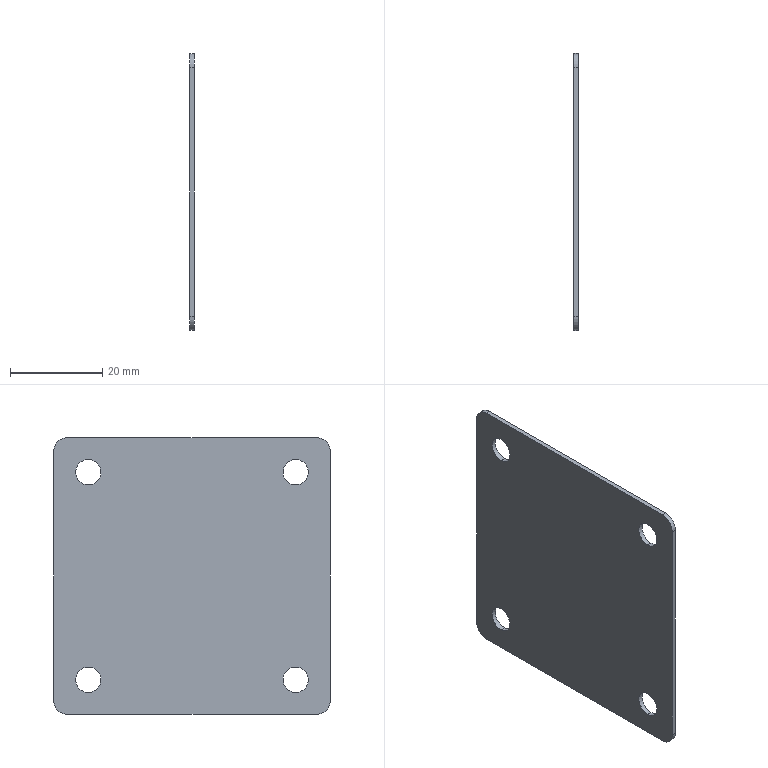Part | STEP file | FFH80-GY-022^FFH85-B3 -02_three-axis module | 1 solid | 18 faces | box 1 x 60 x 60 mm | volume 3497 mm3 | cylinder 12 | plane 6 | commonest cylinder face diameters 5.5 x8 6 x4
STEP:
#1=CARTESIAN_POINT('',(0.,22.5,-19.75));
#2=VERTEX_POINT('',#1);
#3=CARTESIAN_POINT('',(0.,22.5,-25.25));
#4=VERTEX_POINT('',#3);
#5=CARTESIAN_POINT('',(0.,22.5,-22.5));
#6=DIRECTION('',(1.,0.,0.));
#7=DIRECTION('',(0.,0.,-1.));
#8=AXIS2_PLACEMENT_3D('',#5,#6,#7);
#9=CIRCLE('',#8,2.75);
#10=EDGE_CURVE('',#2,#4,#9,.T.);
#11=ORIENTED_EDGE('',*,*,#10,.F.);
#12=CARTESIAN_POINT('',(1.,22.5,-19.75));
#13=VERTEX_POINT('',#12);
#14=CARTESIAN_POINT('',(1.,22.5,-19.75));
#15=DIRECTION('',(1.,0.,0.));
#16=VECTOR('',#15,1000.);
#17=LINE('',#14,#16);
#18=EDGE_CURVE('',#2,#13,#17,.T.);
#19=ORIENTED_EDGE('',*,*,#18,.T.);
#20=CARTESIAN_POINT('',(1.,22.5,-25.25));
#21=VERTEX_POINT('',#20);
#22=CARTESIAN_POINT('',(1.,22.5,-22.5));
#23=DIRECTION('',(1.,0.,0.));
#24=DIRECTION('',(0.,0.,-1.));
#25=AXIS2_PLACEMENT_3D('',#22,#23,#24);
#26=CIRCLE('',#25,2.75);
#27=EDGE_CURVE('',#13,#21,#26,.T.);
#28=ORIENTED_EDGE('',*,*,#27,.T.);
#29=CARTESIAN_POINT('',(1.,22.5,-25.25));
#30=DIRECTION('',(1.,0.,0.));
#31=VECTOR('',#30,1000.);
#32=LINE('',#29,#31);
#33=EDGE_CURVE('',#4,#21,#32,.T.);
#34=ORIENTED_EDGE('',*,*,#33,.F.);
#35=EDGE_LOOP('',(#11,#19,#28,#34));
#36=FACE_OUTER_BOUND('',#35,.T.);
#37=CARTESIAN_POINT('',(1.,22.5,-22.5));
#38=DIRECTION('',(1.,0.,0.));
#39=DIRECTION('',(0.,0.,-1.));
#40=AXIS2_PLACEMENT_3D('',#37,#38,#39);
#41=CYLINDRICAL_SURFACE('',#40,2.75);
#42=ADVANCED_FACE('',(#36),#41,.F.);
#43=CARTESIAN_POINT('',(0.,22.5,25.25));
#44=VERTEX_POINT('',#43);
#45=CARTESIAN_POINT('',(0.,22.5,19.75));
#46=VERTEX_POINT('',#45);
#47=CARTESIAN_POINT('',(0.,22.5,22.5));
#48=DIRECTION('',(1.,0.,0.));
#49=DIRECTION('',(0.,0.,-1.));
#50=AXIS2_PLACEMENT_3D('',#47,#48,#49);
#51=CIRCLE('',#50,2.75);
#52=EDGE_CURVE('',#44,#46,#51,.T.);
#53=ORIENTED_EDGE('',*,*,#52,.F.);
#54=CARTESIAN_POINT('',(1.,22.5,25.25));
#55=VERTEX_POINT('',#54);
#56=CARTESIAN_POINT('',(1.,22.5,25.25));
#57=DIRECTION('',(1.,0.,0.));
#58=VECTOR('',#57,1000.);
#59=LINE('',#56,#58);
#60=EDGE_CURVE('',#44,#55,#59,.T.);
#61=ORIENTED_EDGE('',*,*,#60,.T.);
#62=CARTESIAN_POINT('',(1.,22.5,19.75));
#63=VERTEX_POINT('',#62);
#64=CARTESIAN_POINT('',(1.,22.5,22.5));
#65=DIRECTION('',(1.,0.,0.));
#66=DIRECTION('',(0.,0.,-1.));
#67=AXIS2_PLACEMENT_3D('',#64,#65,#66);
#68=CIRCLE('',#67,2.75);
#69=EDGE_CURVE('',#55,#63,#68,.T.);
#70=ORIENTED_EDGE('',*,*,#69,.T.);
#71=CARTESIAN_POINT('',(1.,22.5,19.75));
#72=DIRECTION('',(1.,0.,0.));
#73=VECTOR('',#72,1000.);
#74=LINE('',#71,#73);
#75=EDGE_CURVE('',#46,#63,#74,.T.);
#76=ORIENTED_EDGE('',*,*,#75,.F.);
#77=EDGE_LOOP('',(#53,#61,#70,#76));
#78=FACE_OUTER_BOUND('',#77,.T.);
#79=CARTESIAN_POINT('',(1.,22.5,22.5));
#80=DIRECTION('',(1.,0.,0.));
#81=DIRECTION('',(0.,0.,-1.));
#82=AXIS2_PLACEMENT_3D('',#79,#80,#81);
#83=CYLINDRICAL_SURFACE('',#82,2.75);
#84=ADVANCED_FACE('',(#78),#83,.F.);
#85=CARTESIAN_POINT('',(0.,-22.5,-19.75));
#86=VERTEX_POINT('',#85);
#87=CARTESIAN_POINT('',(0.,-22.5,-25.25));
#88=VERTEX_POINT('',#87);
#89=CARTESIAN_POINT('',(0.,-22.5,-22.5));
#90=DIRECTION('',(1.,0.,0.));
#91=DIRECTION('',(0.,0.,-1.));
#92=AXIS2_PLACEMENT_3D('',#89,#90,#91);
#93=CIRCLE('',#92,2.75);
#94=EDGE_CURVE('',#86,#88,#93,.T.);
#95=ORIENTED_EDGE('',*,*,#94,.F.);
#96=CARTESIAN_POINT('',(1.,-22.5,-19.75));
#97=VERTEX_POINT('',#96);
#98=CARTESIAN_POINT('',(1.,-22.5,-19.75));
#99=DIRECTION('',(1.,0.,0.));
#100=VECTOR('',#99,1000.);
#101=LINE('',#98,#100);
#102=EDGE_CURVE('',#86,#97,#101,.T.);
#103=ORIENTED_EDGE('',*,*,#102,.T.);
#104=CARTESIAN_POINT('',(1.,-22.5,-25.25));
#105=VERTEX_POINT('',#104);
#106=CARTESIAN_POINT('',(1.,-22.5,-22.5));
#107=DIRECTION('',(1.,0.,0.));
#108=DIRECTION('',(0.,0.,-1.));
#109=AXIS2_PLACEMENT_3D('',#106,#107,#108);
#110=CIRCLE('',#109,2.75);
#111=EDGE_CURVE('',#97,#105,#110,.T.);
#112=ORIENTED_EDGE('',*,*,#111,.T.);
#113=CARTESIAN_POINT('',(1.,-22.5,-25.25));
#114=DIRECTION('',(1.,0.,0.));
#115=VECTOR('',#114,1000.);
#116=LINE('',#113,#115);
#117=EDGE_CURVE('',#88,#105,#116,.T.);
#118=ORIENTED_EDGE('',*,*,#117,.F.);
#119=EDGE_LOOP('',(#95,#103,#112,#118));
#120=FACE_OUTER_BOUND('',#119,.T.);
#121=CARTESIAN_POINT('',(1.,-22.5,-22.5));
#122=DIRECTION('',(1.,0.,0.));
#123=DIRECTION('',(0.,0.,-1.));
#124=AXIS2_PLACEMENT_3D('',#121,#122,#123);
#125=CYLINDRICAL_SURFACE('',#124,2.75);
#126=ADVANCED_FACE('',(#120),#125,.F.);
#127=CARTESIAN_POINT('',(0.,-22.5,25.25));
#128=VERTEX_POINT('',#127);
#129=CARTESIAN_POINT('',(0.,-22.5,19.75));
#130=VERTEX_POINT('',#129);
#131=CARTESIAN_POINT('',(0.,-22.5,22.5));
#132=DIRECTION('',(1.,0.,0.));
#133=DIRECTION('',(0.,0.,-1.));
#134=AXIS2_PLACEMENT_3D('',#131,#132,#133);
#135=CIRCLE('',#134,2.75);
#136=EDGE_CURVE('',#128,#130,#135,.T.);
#137=ORIENTED_EDGE('',*,*,#136,.F.);
#138=CARTESIAN_POINT('',(1.,-22.5,25.25));
#139=VERTEX_POINT('',#138);
#140=CARTESIAN_POINT('',(1.,-22.5,25.25));
#141=DIRECTION('',(1.,0.,0.));
#142=VECTOR('',#141,1000.);
#143=LINE('',#140,#142);
#144=EDGE_CURVE('',#128,#139,#143,.T.);
#145=ORIENTED_EDGE('',*,*,#144,.T.);
#146=CARTESIAN_POINT('',(1.,-22.5,19.75));
#147=VERTEX_POINT('',#146);
#148=CARTESIAN_POINT('',(1.,-22.5,22.5));
#149=DIRECTION('',(1.,0.,0.));
#150=DIRECTION('',(0.,0.,-1.));
#151=AXIS2_PLACEMENT_3D('',#148,#149,#150);
#152=CIRCLE('',#151,2.75);
#153=EDGE_CURVE('',#139,#147,#152,.T.);
#154=ORIENTED_EDGE('',*,*,#153,.T.);
#155=CARTESIAN_POINT('',(1.,-22.5,19.75));
#156=DIRECTION('',(1.,0.,0.));
#157=VECTOR('',#156,1000.);
#158=LINE('',#155,#157);
#159=EDGE_CURVE('',#130,#147,#158,.T.);
#160=ORIENTED_EDGE('',*,*,#159,.F.);
#161=EDGE_LOOP('',(#137,#145,#154,#160));
#162=FACE_OUTER_BOUND('',#161,.T.);
#163=CARTESIAN_POINT('',(1.,-22.5,22.5));
#164=DIRECTION('',(1.,0.,0.));
#165=DIRECTION('',(0.,0.,-1.));
#166=AXIS2_PLACEMENT_3D('',#163,#164,#165);
#167=CYLINDRICAL_SURFACE('',#166,2.75);
#168=ADVANCED_FACE('',(#162),#167,.F.);
#169=CARTESIAN_POINT('',(1.,22.5,-22.5));
#170=DIRECTION('',(1.,0.,0.));
#171=DIRECTION('',(0.,0.,-1.));
#172=AXIS2_PLACEMENT_3D('',#169,#170,#171);
#173=CIRCLE('',#172,2.75);
#174=EDGE_CURVE('',#21,#13,#173,.T.);
#175=ORIENTED_EDGE('',*,*,#174,.F.);
#176=ORIENTED_EDGE('',*,*,#27,.F.);
#177=EDGE_LOOP('',(#175,#176));
#178=FACE_BOUND('',#177,.T.);
#179=CARTESIAN_POINT('',(1.,22.5,22.5));
#180=DIRECTION('',(1.,0.,0.));
#181=DIRECTION('',(0.,0.,-1.));
#182=AXIS2_PLACEMENT_3D('',#179,#180,#181);
#183=CIRCLE('',#182,2.75);
#184=EDGE_CURVE('',#63,#55,#183,.T.);
#185=ORIENTED_EDGE('',*,*,#184,.F.);
#186=ORIENTED_EDGE('',*,*,#69,.F.);
#187=EDGE_LOOP('',(#185,#186));
#188=FACE_BOUND('',#187,.T.);
#189=CARTESIAN_POINT('',(1.,-22.5,-22.5));
#190=DIRECTION('',(1.,0.,0.));
#191=DIRECTION('',(0.,0.,-1.));
#192=AXIS2_PLACEMENT_3D('',#189,#190,#191);
#193=CIRCLE('',#192,2.75);
#194=EDGE_CURVE('',#105,#97,#193,.T.);
#195=ORIENTED_EDGE('',*,*,#194,.F.);
#196=ORIENTED_EDGE('',*,*,#111,.F.);
#197=EDGE_LOOP('',(#195,#196));
#198=FACE_BOUND('',#197,.T.);
#199=CARTESIAN_POINT('',(1.,-22.5,22.5));
#200=DIRECTION('',(1.,0.,0.));
#201=DIRECTION('',(0.,0.,-1.));
#202=AXIS2_PLACEMENT_3D('',#199,#200,#201);
#203=CIRCLE('',#202,2.75);
#204=EDGE_CURVE('',#147,#139,#203,.T.);
#205=ORIENTED_EDGE('',*,*,#204,.F.);
#206=ORIENTED_EDGE('',*,*,#153,.F.);
#207=EDGE_LOOP('',(#205,#206));
#208=FACE_BOUND('',#207,.T.);
#209=CARTESIAN_POINT('',(1.,-30.,-27.));
#210=VERTEX_POINT('',#209);
#211=CARTESIAN_POINT('',(1.,-30.,27.));
#212=VERTEX_POINT('',#211);
#213=CARTESIAN_POINT('',(1.,-30.,0.));
#214=DIRECTION('',(0.,0.,1.));
#215=VECTOR('',#214,1000.);
#216=LINE('',#213,#215);
#217=EDGE_CURVE('',#210,#212,#216,.T.);
#218=ORIENTED_EDGE('',*,*,#217,.F.);
#219=CARTESIAN_POINT('',(1.,-27.,-30.));
#220=VERTEX_POINT('',#219);
#221=CARTESIAN_POINT('',(1.,-27.,-27.));
#222=DIRECTION('',(-1.,0.,0.));
#223=DIRECTION('',(0.,0.,1.));
#224=AXIS2_PLACEMENT_3D('',#221,#222,#223);
#225=CIRCLE('',#224,3.);
#226=EDGE_CURVE('',#220,#210,#225,.T.);
#227=ORIENTED_EDGE('',*,*,#226,.F.);
#228=CARTESIAN_POINT('',(1.,27.,-30.));
#229=VERTEX_POINT('',#228);
#230=CARTESIAN_POINT('',(1.,0.,-30.));
#231=DIRECTION('',(0.,-1.,0.));
#232=VECTOR('',#231,1000.);
#233=LINE('',#230,#232);
#234=EDGE_CURVE('',#229,#220,#233,.T.);
#235=ORIENTED_EDGE('',*,*,#234,.F.);
#236=CARTESIAN_POINT('',(1.,30.,-27.));
#237=VERTEX_POINT('',#236);
#238=CARTESIAN_POINT('',(1.,27.,-27.));
#239=DIRECTION('',(-1.,0.,0.));
#240=DIRECTION('',(0.,0.,1.));
#241=AXIS2_PLACEMENT_3D('',#238,#239,#240);
#242=CIRCLE('',#241,3.);
#243=EDGE_CURVE('',#237,#229,#242,.T.);
#244=ORIENTED_EDGE('',*,*,#243,.F.);
#245=CARTESIAN_POINT('',(1.,30.,27.));
#246=VERTEX_POINT('',#245);
#247=CARTESIAN_POINT('',(1.,30.,0.));
#248=DIRECTION('',(0.,0.,-1.));
#249=VECTOR('',#248,1000.);
#250=LINE('',#247,#249);
#251=EDGE_CURVE('',#246,#237,#250,.T.);
#252=ORIENTED_EDGE('',*,*,#251,.F.);
#253=CARTESIAN_POINT('',(1.,27.,30.));
#254=VERTEX_POINT('',#253);
#255=CARTESIAN_POINT('',(1.,27.,27.));
#256=DIRECTION('',(-1.,0.,0.));
#257=DIRECTION('',(0.,0.,1.));
#258=AXIS2_PLACEMENT_3D('',#255,#256,#257);
#259=CIRCLE('',#258,3.);
#260=EDGE_CURVE('',#254,#246,#259,.T.);
#261=ORIENTED_EDGE('',*,*,#260,.F.);
#262=CARTESIAN_POINT('',(1.,-27.,30.));
#263=VERTEX_POINT('',#262);
#264=CARTESIAN_POINT('',(1.,0.,30.));
#265=DIRECTION('',(0.,1.,0.));
#266=VECTOR('',#265,1000.);
#267=LINE('',#264,#266);
#268=EDGE_CURVE('',#263,#254,#267,.T.);
#269=ORIENTED_EDGE('',*,*,#268,.F.);
#270=CARTESIAN_POINT('',(1.,-27.,27.));
#271=DIRECTION('',(-1.,0.,0.));
#272=DIRECTION('',(0.,0.,1.));
#273=AXIS2_PLACEMENT_3D('',#270,#271,#272);
#274=CIRCLE('',#273,3.);
#275=EDGE_CURVE('',#212,#263,#274,.T.);
#276=ORIENTED_EDGE('',*,*,#275,.F.);
#277=EDGE_LOOP('',(#218,#227,#235,#244,#252,#261,#269,#276));
#278=FACE_OUTER_BOUND('',#277,.T.);
#279=CARTESIAN_POINT('',(1.,0.,0.));
#280=DIRECTION('',(-1.,0.,0.));
#281=DIRECTION('',(0.,0.,1.));
#282=AXIS2_PLACEMENT_3D('',#279,#280,#281);
#283=PLANE('',#282);
#284=ADVANCED_FACE('',(#178,#188,#198,#208,#278),#283,.F.);
#285=ORIENTED_EDGE('',*,*,#18,.F.);
#286=CARTESIAN_POINT('',(0.,22.5,-22.5));
#287=DIRECTION('',(1.,0.,0.));
#288=DIRECTION('',(0.,0.,-1.));
#289=AXIS2_PLACEMENT_3D('',#286,#287,#288);
#290=CIRCLE('',#289,2.75);
#291=EDGE_CURVE('',#4,#2,#290,.T.);
#292=ORIENTED_EDGE('',*,*,#291,.F.);
#293=ORIENTED_EDGE('',*,*,#33,.T.);
#294=ORIENTED_EDGE('',*,*,#174,.T.);
#295=EDGE_LOOP('',(#285,#292,#293,#294));
#296=FACE_OUTER_BOUND('',#295,.T.);
#297=CARTESIAN_POINT('',(1.,22.5,-22.5));
#298=DIRECTION('',(1.,0.,0.));
#299=DIRECTION('',(0.,0.,-1.));
#300=AXIS2_PLACEMENT_3D('',#297,#298,#299);
#301=CYLINDRICAL_SURFACE('',#300,2.75);
#302=ADVANCED_FACE('',(#296),#301,.F.);
#303=ORIENTED_EDGE('',*,*,#60,.F.);
#304=CARTESIAN_POINT('',(0.,22.5,22.5));
#305=DIRECTION('',(1.,0.,0.));
#306=DIRECTION('',(0.,0.,-1.));
#307=AXIS2_PLACEMENT_3D('',#304,#305,#306);
#308=CIRCLE('',#307,2.75);
#309=EDGE_CURVE('',#46,#44,#308,.T.);
#310=ORIENTED_EDGE('',*,*,#309,.F.);
#311=ORIENTED_EDGE('',*,*,#75,.T.);
#312=ORIENTED_EDGE('',*,*,#184,.T.);
#313=EDGE_LOOP('',(#303,#310,#311,#312));
#314=FACE_OUTER_BOUND('',#313,.T.);
#315=CARTESIAN_POINT('',(1.,22.5,22.5));
#316=DIRECTION('',(1.,0.,0.));
#317=DIRECTION('',(0.,0.,-1.));
#318=AXIS2_PLACEMENT_3D('',#315,#316,#317);
#319=CYLINDRICAL_SURFACE('',#318,2.75);
#320=ADVANCED_FACE('',(#314),#319,.F.);
#321=ORIENTED_EDGE('',*,*,#102,.F.);
#322=CARTESIAN_POINT('',(0.,-22.5,-22.5));
#323=DIRECTION('',(1.,0.,0.));
#324=DIRECTION('',(0.,0.,-1.));
#325=AXIS2_PLACEMENT_3D('',#322,#323,#324);
#326=CIRCLE('',#325,2.75);
#327=EDGE_CURVE('',#88,#86,#326,.T.);
#328=ORIENTED_EDGE('',*,*,#327,.F.);
#329=ORIENTED_EDGE('',*,*,#117,.T.);
#330=ORIENTED_EDGE('',*,*,#194,.T.);
#331=EDGE_LOOP('',(#321,#328,#329,#330));
#332=FACE_OUTER_BOUND('',#331,.T.);
#333=CARTESIAN_POINT('',(1.,-22.5,-22.5));
#334=DIRECTION('',(1.,0.,0.));
#335=DIRECTION('',(0.,0.,-1.));
#336=AXIS2_PLACEMENT_3D('',#333,#334,#335);
#337=CYLINDRICAL_SURFACE('',#336,2.75);
#338=ADVANCED_FACE('',(#332),#337,.F.);
#339=ORIENTED_EDGE('',*,*,#144,.F.);
#340=CARTESIAN_POINT('',(0.,-22.5,22.5));
#341=DIRECTION('',(1.,0.,0.));
#342=DIRECTION('',(0.,0.,-1.));
#343=AXIS2_PLACEMENT_3D('',#340,#341,#342);
#344=CIRCLE('',#343,2.75);
#345=EDGE_CURVE('',#130,#128,#344,.T.);
#346=ORIENTED_EDGE('',*,*,#345,.F.);
#347=ORIENTED_EDGE('',*,*,#159,.T.);
#348=ORIENTED_EDGE('',*,*,#204,.T.);
#349=EDGE_LOOP('',(#339,#346,#347,#348));
#350=FACE_OUTER_BOUND('',#349,.T.);
#351=CARTESIAN_POINT('',(1.,-22.5,22.5));
#352=DIRECTION('',(1.,0.,0.));
#353=DIRECTION('',(0.,0.,-1.));
#354=AXIS2_PLACEMENT_3D('',#351,#352,#353);
#355=CYLINDRICAL_SURFACE('',#354,2.75);
#356=ADVANCED_FACE('',(#350),#355,.F.);
#357=ORIENTED_EDGE('',*,*,#275,.T.);
#358=CARTESIAN_POINT('',(0.,-27.,30.));
#359=VERTEX_POINT('',#358);
#360=CARTESIAN_POINT('',(1.,-27.,30.));
#361=DIRECTION('',(-1.,0.,0.));
#362=VECTOR('',#361,1000.);
#363=LINE('',#360,#362);
#364=EDGE_CURVE('',#263,#359,#363,.T.);
#365=ORIENTED_EDGE('',*,*,#364,.T.);
#366=CARTESIAN_POINT('',(0.,-30.,27.));
#367=VERTEX_POINT('',#366);
#368=CARTESIAN_POINT('',(0.,-27.,27.));
#369=DIRECTION('',(1.,0.,0.));
#370=DIRECTION('',(0.,0.,1.));
#371=AXIS2_PLACEMENT_3D('',#368,#369,#370);
#372=CIRCLE('',#371,3.);
#373=EDGE_CURVE('',#359,#367,#372,.T.);
#374=ORIENTED_EDGE('',*,*,#373,.T.);
#375=CARTESIAN_POINT('',(1.,-30.,27.));
#376=DIRECTION('',(1.,0.,0.));
#377=VECTOR('',#376,1000.);
#378=LINE('',#375,#377);
#379=EDGE_CURVE('',#367,#212,#378,.T.);
#380=ORIENTED_EDGE('',*,*,#379,.T.);
#381=EDGE_LOOP('',(#357,#365,#374,#380));
#382=FACE_OUTER_BOUND('',#381,.T.);
#383=CARTESIAN_POINT('',(1.,-27.,27.));
#384=DIRECTION('',(-1.,0.,0.));
#385=DIRECTION('',(0.,0.,1.));
#386=AXIS2_PLACEMENT_3D('',#383,#384,#385);
#387=CYLINDRICAL_SURFACE('',#386,3.);
#388=ADVANCED_FACE('',(#382),#387,.T.);
#389=CARTESIAN_POINT('',(0.,-30.,-27.));
#390=VERTEX_POINT('',#389);
#391=CARTESIAN_POINT('',(0.,-30.,-30.));
#392=DIRECTION('',(0.,0.,1.));
#393=VECTOR('',#392,1000.);
#394=LINE('',#391,#393);
#395=EDGE_CURVE('',#390,#367,#394,.T.);
#396=ORIENTED_EDGE('',*,*,#395,.F.);
#397=CARTESIAN_POINT('',(1.,-30.,-27.));
#398=DIRECTION('',(-1.,0.,0.));
#399=VECTOR('',#398,1000.);
#400=LINE('',#397,#399);
#401=EDGE_CURVE('',#210,#390,#400,.T.);
#402=ORIENTED_EDGE('',*,*,#401,.F.);
#403=ORIENTED_EDGE('',*,*,#217,.T.);
#404=ORIENTED_EDGE('',*,*,#379,.F.);
#405=EDGE_LOOP('',(#396,#402,#403,#404));
#406=FACE_OUTER_BOUND('',#405,.T.);
#407=CARTESIAN_POINT('',(1.,-30.,-30.));
#408=DIRECTION('',(0.,1.,0.));
#409=DIRECTION('',(0.,0.,1.));
#410=AXIS2_PLACEMENT_3D('',#407,#408,#409);
#411=PLANE('',#410);
#412=ADVANCED_FACE('',(#406),#411,.F.);
#413=ORIENTED_EDGE('',*,*,#226,.T.);
#414=ORIENTED_EDGE('',*,*,#401,.T.);
#415=CARTESIAN_POINT('',(0.,-27.,-30.));
#416=VERTEX_POINT('',#415);
#417=CARTESIAN_POINT('',(0.,-27.,-27.));
#418=DIRECTION('',(1.,0.,0.));
#419=DIRECTION('',(0.,0.,1.));
#420=AXIS2_PLACEMENT_3D('',#417,#418,#419);
#421=CIRCLE('',#420,3.);
#422=EDGE_CURVE('',#390,#416,#421,.T.);
#423=ORIENTED_EDGE('',*,*,#422,.T.);
#424=CARTESIAN_POINT('',(1.,-27.,-30.));
#425=DIRECTION('',(1.,0.,0.));
#426=VECTOR('',#425,1000.);
#427=LINE('',#424,#426);
#428=EDGE_CURVE('',#416,#220,#427,.T.);
#429=ORIENTED_EDGE('',*,*,#428,.T.);
#430=EDGE_LOOP('',(#413,#414,#423,#429));
#431=FACE_OUTER_BOUND('',#430,.T.);
#432=CARTESIAN_POINT('',(1.,-27.,-27.));
#433=DIRECTION('',(-1.,0.,0.));
#434=DIRECTION('',(0.,0.,1.));
#435=AXIS2_PLACEMENT_3D('',#432,#433,#434);
#436=CYLINDRICAL_SURFACE('',#435,3.);
#437=ADVANCED_FACE('',(#431),#436,.T.);
#438=CARTESIAN_POINT('',(0.,27.,-30.));
#439=VERTEX_POINT('',#438);
#440=CARTESIAN_POINT('',(0.,30.,-30.));
#441=DIRECTION('',(0.,-1.,0.));
#442=VECTOR('',#441,1000.);
#443=LINE('',#440,#442);
#444=EDGE_CURVE('',#439,#416,#443,.T.);
#445=ORIENTED_EDGE('',*,*,#444,.F.);
#446=CARTESIAN_POINT('',(1.,27.,-30.));
#447=DIRECTION('',(-1.,0.,0.));
#448=VECTOR('',#447,1000.);
#449=LINE('',#446,#448);
#450=EDGE_CURVE('',#229,#439,#449,.T.);
#451=ORIENTED_EDGE('',*,*,#450,.F.);
#452=ORIENTED_EDGE('',*,*,#234,.T.);
#453=ORIENTED_EDGE('',*,*,#428,.F.);
#454=EDGE_LOOP('',(#445,#451,#452,#453));
#455=FACE_OUTER_BOUND('',#454,.T.);
#456=CARTESIAN_POINT('',(1.,30.,-30.));
#457=DIRECTION('',(0.,0.,1.));
#458=DIRECTION('',(0.,-1.,0.));
#459=AXIS2_PLACEMENT_3D('',#456,#457,#458);
#460=PLANE('',#459);
#461=ADVANCED_FACE('',(#455),#460,.F.);
#462=ORIENTED_EDGE('',*,*,#243,.T.);
#463=ORIENTED_EDGE('',*,*,#450,.T.);
#464=CARTESIAN_POINT('',(0.,30.,-27.));
#465=VERTEX_POINT('',#464);
#466=CARTESIAN_POINT('',(0.,27.,-27.));
#467=DIRECTION('',(1.,0.,0.));
#468=DIRECTION('',(0.,0.,1.));
#469=AXIS2_PLACEMENT_3D('',#466,#467,#468);
#470=CIRCLE('',#469,3.);
#471=EDGE_CURVE('',#439,#465,#470,.T.);
#472=ORIENTED_EDGE('',*,*,#471,.T.);
#473=CARTESIAN_POINT('',(1.,30.,-27.));
#474=DIRECTION('',(1.,0.,0.));
#475=VECTOR('',#474,1000.);
#476=LINE('',#473,#475);
#477=EDGE_CURVE('',#465,#237,#476,.T.);
#478=ORIENTED_EDGE('',*,*,#477,.T.);
#479=EDGE_LOOP('',(#462,#463,#472,#478));
#480=FACE_OUTER_BOUND('',#479,.T.);
#481=CARTESIAN_POINT('',(1.,27.,-27.));
#482=DIRECTION('',(-1.,0.,0.));
#483=DIRECTION('',(0.,0.,1.));
#484=AXIS2_PLACEMENT_3D('',#481,#482,#483);
#485=CYLINDRICAL_SURFACE('',#484,3.);
#486=ADVANCED_FACE('',(#480),#485,.T.);
#487=CARTESIAN_POINT('',(0.,30.,27.));
#488=VERTEX_POINT('',#487);
#489=CARTESIAN_POINT('',(0.,30.,-30.));
#490=DIRECTION('',(0.,0.,-1.));
#491=VECTOR('',#490,1000.);
#492=LINE('',#489,#491);
#493=EDGE_CURVE('',#488,#465,#492,.T.);
#494=ORIENTED_EDGE('',*,*,#493,.F.);
#495=CARTESIAN_POINT('',(1.,30.,27.));
#496=DIRECTION('',(-1.,0.,0.));
#497=VECTOR('',#496,1000.);
#498=LINE('',#495,#497);
#499=EDGE_CURVE('',#246,#488,#498,.T.);
#500=ORIENTED_EDGE('',*,*,#499,.F.);
#501=ORIENTED_EDGE('',*,*,#251,.T.);
#502=ORIENTED_EDGE('',*,*,#477,.F.);
#503=EDGE_LOOP('',(#494,#500,#501,#502));
#504=FACE_OUTER_BOUND('',#503,.T.);
#505=CARTESIAN_POINT('',(1.,30.,-30.));
#506=DIRECTION('',(0.,-1.,0.));
#507=DIRECTION('',(0.,0.,-1.));
#508=AXIS2_PLACEMENT_3D('',#505,#506,#507);
#509=PLANE('',#508);
#510=ADVANCED_FACE('',(#504),#509,.F.);
#511=ORIENTED_EDGE('',*,*,#260,.T.);
#512=ORIENTED_EDGE('',*,*,#499,.T.);
#513=CARTESIAN_POINT('',(0.,27.,30.));
#514=VERTEX_POINT('',#513);
#515=CARTESIAN_POINT('',(0.,27.,27.));
#516=DIRECTION('',(1.,0.,0.));
#517=DIRECTION('',(0.,0.,1.));
#518=AXIS2_PLACEMENT_3D('',#515,#516,#517);
#519=CIRCLE('',#518,3.);
#520=EDGE_CURVE('',#488,#514,#519,.T.);
#521=ORIENTED_EDGE('',*,*,#520,.T.);
#522=CARTESIAN_POINT('',(1.,27.,30.));
#523=DIRECTION('',(1.,0.,0.));
#524=VECTOR('',#523,1000.);
#525=LINE('',#522,#524);
#526=EDGE_CURVE('',#514,#254,#525,.T.);
#527=ORIENTED_EDGE('',*,*,#526,.T.);
#528=EDGE_LOOP('',(#511,#512,#521,#527));
#529=FACE_OUTER_BOUND('',#528,.T.);
#530=CARTESIAN_POINT('',(1.,27.,27.));
#531=DIRECTION('',(-1.,0.,0.));
#532=DIRECTION('',(0.,0.,1.));
#533=AXIS2_PLACEMENT_3D('',#530,#531,#532);
#534=CYLINDRICAL_SURFACE('',#533,3.);
#535=ADVANCED_FACE('',(#529),#534,.T.);
#536=ORIENTED_EDGE('',*,*,#268,.T.);
#537=ORIENTED_EDGE('',*,*,#526,.F.);
#538=CARTESIAN_POINT('',(0.,30.,30.));
#539=DIRECTION('',(0.,1.,0.));
#540=VECTOR('',#539,1000.);
#541=LINE('',#538,#540);
#542=EDGE_CURVE('',#359,#514,#541,.T.);
#543=ORIENTED_EDGE('',*,*,#542,.F.);
#544=ORIENTED_EDGE('',*,*,#364,.F.);
#545=EDGE_LOOP('',(#536,#537,#543,#544));
#546=FACE_OUTER_BOUND('',#545,.T.);
#547=CARTESIAN_POINT('',(1.,30.,30.));
#548=DIRECTION('',(0.,0.,-1.));
#549=DIRECTION('',(0.,1.,0.));
#550=AXIS2_PLACEMENT_3D('',#547,#548,#549);
#551=PLANE('',#550);
#552=ADVANCED_FACE('',(#546),#551,.F.);
#553=ORIENTED_EDGE('',*,*,#291,.T.);
#554=ORIENTED_EDGE('',*,*,#10,.T.);
#555=EDGE_LOOP('',(#553,#554));
#556=FACE_BOUND('',#555,.T.);
#557=ORIENTED_EDGE('',*,*,#309,.T.);
#558=ORIENTED_EDGE('',*,*,#52,.T.);
#559=EDGE_LOOP('',(#557,#558));
#560=FACE_BOUND('',#559,.T.);
#561=ORIENTED_EDGE('',*,*,#327,.T.);
#562=ORIENTED_EDGE('',*,*,#94,.T.);
#563=EDGE_LOOP('',(#561,#562));
#564=FACE_BOUND('',#563,.T.);
#565=ORIENTED_EDGE('',*,*,#345,.T.);
#566=ORIENTED_EDGE('',*,*,#136,.T.);
#567=EDGE_LOOP('',(#565,#566));
#568=FACE_BOUND('',#567,.T.);
#569=ORIENTED_EDGE('',*,*,#493,.T.);
#570=ORIENTED_EDGE('',*,*,#471,.F.);
#571=ORIENTED_EDGE('',*,*,#444,.T.);
#572=ORIENTED_EDGE('',*,*,#422,.F.);
#573=ORIENTED_EDGE('',*,*,#395,.T.);
#574=ORIENTED_EDGE('',*,*,#373,.F.);
#575=ORIENTED_EDGE('',*,*,#542,.T.);
#576=ORIENTED_EDGE('',*,*,#520,.F.);
#577=EDGE_LOOP('',(#569,#570,#571,#572,#573,#574,#575,#576));
#578=FACE_OUTER_BOUND('',#577,.T.);
#579=CARTESIAN_POINT('',(0.,0.,0.));
#580=DIRECTION('',(-1.,0.,0.));
#581=DIRECTION('',(0.,0.,1.));
#582=AXIS2_PLACEMENT_3D('',#579,#580,#581);
#583=PLANE('',#582);
#584=ADVANCED_FACE('',(#556,#560,#564,#568,#578),#583,.T.);
#585=CLOSED_SHELL('',(#42,#84,#126,#168,#284,#302,#320,#338,#356,#388,#412,#437,#461,#486,#510,#535,#552,#584));
#586=MANIFOLD_SOLID_BREP('',#585);
#587=CARTESIAN_POINT('',(0.,0.,0.));
#588=DIRECTION('',(0.,0.,1.));
#589=DIRECTION('',(1.,0.,0.));
#590=AXIS2_PLACEMENT_3D('',#587,#588,#589);
#591=(LENGTH_UNIT()NAMED_UNIT(*)SI_UNIT(.MILLI.,.METRE.));
#592=UNCERTAINTY_MEASURE_WITH_UNIT(LENGTH_MEASURE(0.00001),#591,'','');
#593=(NAMED_UNIT(*)PLANE_ANGLE_UNIT()SI_UNIT($,.RADIAN.));
#594=(NAMED_UNIT(*)SI_UNIT($,.STERADIAN.)SOLID_ANGLE_UNIT());
#595=(GEOMETRIC_REPRESENTATION_CONTEXT(3)GLOBAL_UNCERTAINTY_ASSIGNED_CONTEXT((#592))GLOBAL_UNIT_ASSIGNED_CONTEXT((#591,#593,#594))REPRESENTATION_CONTEXT('',''));
#596=ADVANCED_BREP_SHAPE_REPRESENTATION('',(#586,#590),#595);